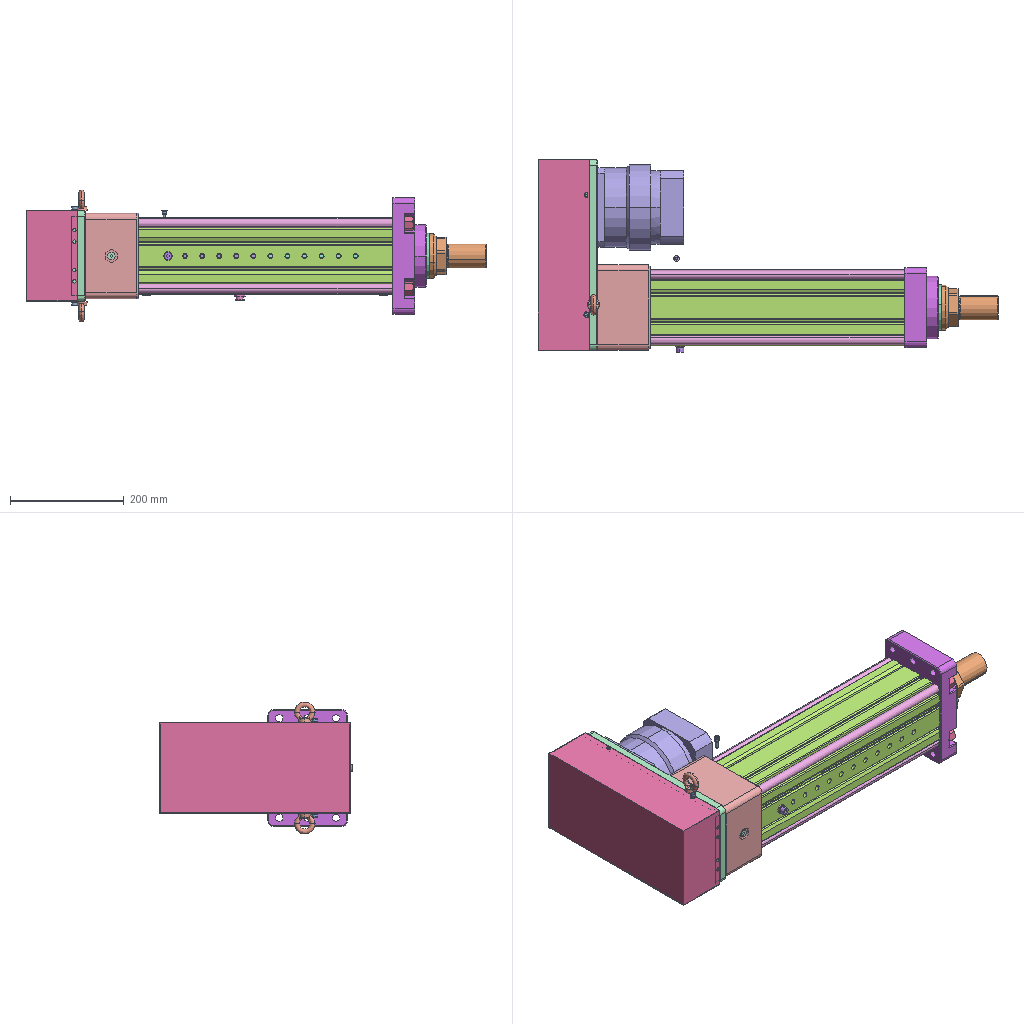Assembly | SolidWorks | 35 different items | 52 placed | box 809 x 339 x 232 mm
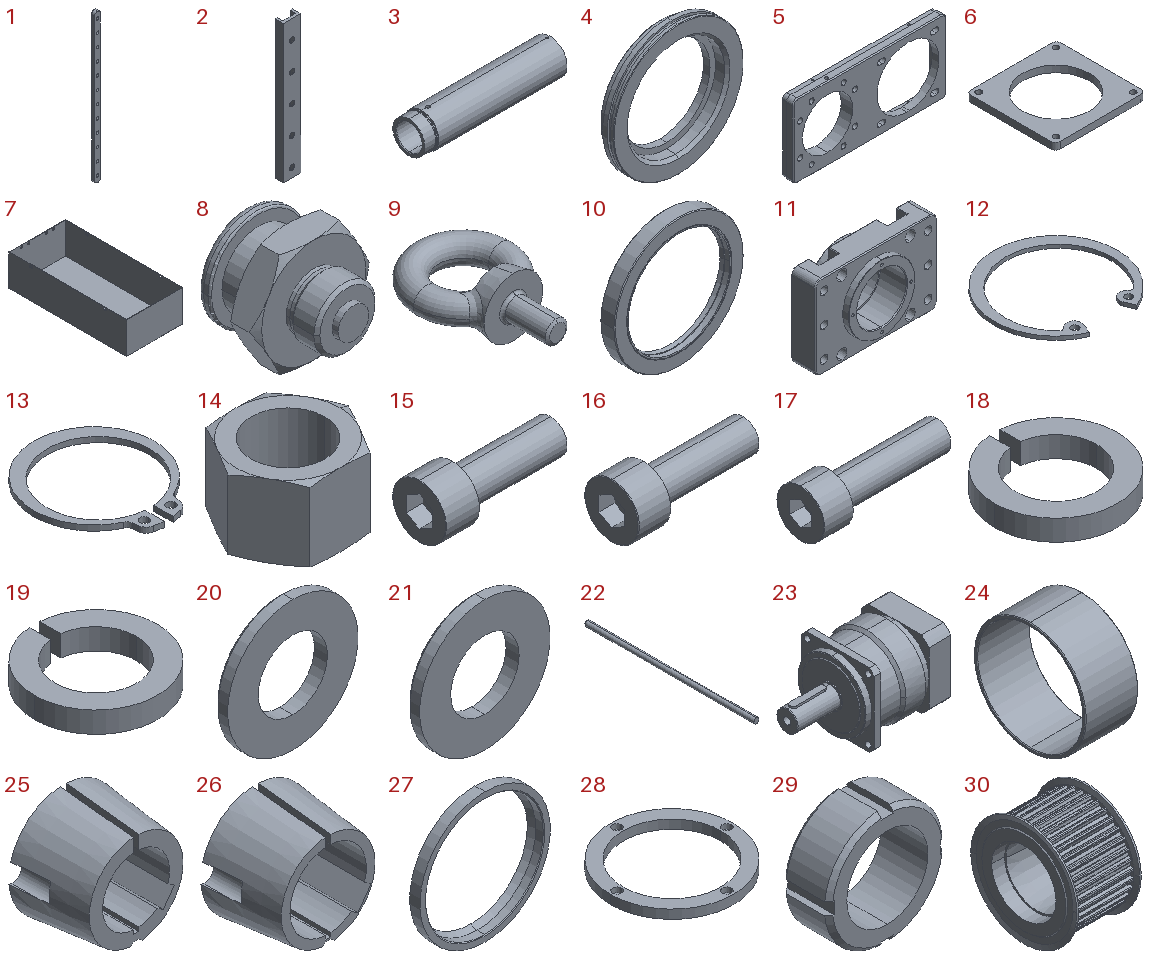Parts list (item | name | quantity | size | volume | features):
1 | - | x1 | 14 x 8 x 360 mm | 35757 mm3 | features ICE 2, Extrusion 1, Fillet 1, HoleWzd 1, LPattern 1
2 | - | x1 | 19 x 9 x 150 mm | 12195 mm3 | features Chamfer 1, Extrusion 1, HoleWzd 1, LPattern 1
3 | - | x1 | 330.5 x 80 x 80 mm | 682443 mm3 | features ICE 3, Chamfer 2, HoleWzd 1, Revolution 1
4 | - | x1 | 120 x 17 x 120 mm | 76412 mm3 | features ICE 4, Chamfer 3, Extrusion 1, MoveFace 1
5 | - | x1 | 335 x 25 x 160 mm | 627344 mm3 | features HoleWzd 7, ICE 6, MoveFace 4, Fillet 2, MirrorPattern 2, Chamfer 1, Extrusion 1
6 | - | x1 | 137 x 135 x 10 mm | 103302 mm3 | features HoleWzd 2, Extrusion 1, Fillet 1, ICE 1, MoveFace 1
7 | - | x1 | 160 x 335 x 90 mm | 168968 mm3 | features ICE 2, Extrusion 1, Shell 1
8 | - | x1 | 19.63 x 18 x 17 mm | 2444 mm3 | features ICE 3, Revolution 2
9 | - | x2 | 36.2 x 52.1 x 21.1 mm | 7704 mm3 | features Fillet 2, Extrusion 1, LPattern 1, RevCut 1, Revolution 1, Sweep 1
10 | - | x1 | 90 x 10 x 90 mm | 7063 mm3 | features BaseBody 1
11 | - | x1 | 205 x 70 x 140 mm | 920988 mm3 | features ICE 17, HoleWzd 12, Chamfer 11, Fillet 5, CirPattern 4, Extrusion 1, MirrorPattern 1, MoveFace 1, RevCut 1
12 | - | x1 | 50.5 x 48.578 x 1.5 mm | 759.16 mm3 | features Extrusion 1
13 | - | x1 | 27.3 x 30.557 x 1.2 mm | 213.948 mm3 | features Extrusion 1, Fillet 1
14 | - | x4 | 26.17 x 22.664 x 15.9 mm | 3864 mm3 | features Cut 2, Chamfer 1, Extrusion 1
15 | - | x2 | 40 x 16 x 16 mm | 4081 mm3 | features BlendCut 1, Cut 1, Fillet 1, LPattern 1, RevCut 1, Revolution 1
16 | - | x3 | 21 x 8.5 x 8.5 mm | 561.928 mm3 | features BlendCut 1, Cut 1, Fillet 1, LPattern 1, RevCut 1, Revolution 1
17 | - | x1 | 38 x 13 x 13 mm | 2440 mm3 | features BlendCut 1, Cut 1, Fillet 1, LPattern 1, RevCut 1, Revolution 1
18 | - | x3 | 7.686 x 7.672 x 1.3 mm | 32.664 mm3 | features Extrusion 1
19 | - | x1 | 12.277 x 12.254 x 2.1 mm | 135.755 mm3 | features Extrusion 1
20 | - | x3 | 10 x 1 x 10 mm | 55.513 mm3 | features Revolution 1
21 | - | x1 | 16 x 1.6 x 16 mm | 229.077 mm3 | features Revolution 1
22 | - | x4 | 16 x 531.5 x 16 mm | 106666 mm3 | features Chamfer 1, Extrusion 1
23 | - | x1 | 248.5 x 150 x 150 mm | 2601531 mm3 | features BaseBody 1
24 | - | x1 | 40 x 85 x 85 mm | 25789 mm3 | features Chamfer 3, MoveFace 1, Revolution 1
25 | - | x1 | 56.795 x 38 x 56.678 mm | 42357 mm3 | features BaseBody 1, ICE 1
26 | - | x1 | 56.795 x 38 x 56.678 mm | 31152 mm3 | features BaseBody 1, ICE 1
27 | - | x1 | 90 x 9.8 x 90 mm | 9491 mm3 | features Chamfer 1, Revolution 1
28 | - | x1 | 111 x 111 x 8 mm | 27617 mm3 | features CirPattern 1, Extrusion 1, HoleWzd 1
29 | - | x1 | 57.689 x 23 x 57.689 mm | 29622 mm3 | features Chamfer 1, CirPattern 1, Extrusion 1, ICE 1
30 | - | x2 | 60 x 99 x 99 mm | 224539 mm3 | features ICE 4, Revolution 2, Chamfer 1, CirPattern 1, MirrorPattern 1
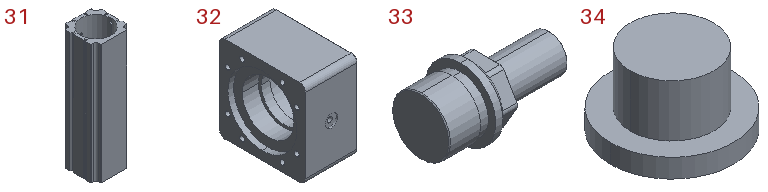31 | - | x1 | 134 x 134 x 446.5 mm | 2883696 mm3 | features ICE 6, HoleWzd 5, Chamfer 3, CirPattern 3, Fillet 3, LPattern 2, MirrorPattern 2, Extrusion 1, MoveFace 1
32 | - | x1 | 99 x 150 x 150 mm | 1431839 mm3 | features ICE 13, HoleWzd 4, Chamfer 2, CirPattern 1, Extrusion 1, Fillet 1
33 | - | x1 | 145 x 79 x 79 mm | 357004 mm3 | features ICE 7, Chamfer 6, Draft 2, Extrusion 1, Fillet 1, MoveFace 1
34 | - | x3 | 13 x 13 x 7.5 mm | 544.556 mm3 | features ICE 2, Extrusion 1
35 | hexagon socket countersunk head screws gb | x1 | - | - | -
Mates (type | each side: item.copy, entity, surface, feature):
Coincident | 32.1 plane | assembly plane | 2 times
Coincident | 32.1 face plane Boss-Extrude1 | 31.1 face plane Boss-Extrude1
Concentric | 32.1 face cylinder M16 Tapped Hole1 | 22.1 face cylinder Boss-Extrude1
Tangent | 31.1 face cylinder Boss-Extrude1 | 1.1 face plane Boss-Extrude1
Concentric | 31.1 face cylinder Ø9.0 (9) Diameter Hole1 | 1.1 face cylinder M8 Tapped Hole1
Coincident | 32.1 face plane Cut-Extrude9 | 28.1 face plane Boss-Extrude1
Concentric | 32.1 face cylinder M4 Tapped Hole2 | 28.1 face cylinder Hole size per socket head cap screw type 1
Concentric | 22.1 face cylinder Boss-Extrude1 | 14.1 face cylinder Base-Extrude
Concentric | 22.1 face cylinder Boss-Extrude1 | 11.1 face cylinder Hole size per socket head cap screw type 1
Coincident | 31.1 face plane Boss-Extrude1 | 11.1 face plane Boss-Extrude1
Concentric | 24.1 face cylinder Revolve1 | 11.1 face cylinder Cut-Extrude11
Coincident | 24.1 face plane Revolve1 | 11.1 face plane Cut-Extrude2
Concentric | 27.1 face cylinder Base-Revolve | 11.1 face cylinder Cut-Revolve2
Coincident | 27.1 face plane Base-Revolve | 11.1 face plane Cut-Revolve2
Concentric | 22.2 face cylinder Boss-Extrude1 | 11.1 face cylinder Hole size per socket head cap screw type 1
Coincident | 22.1 face plane Boss-Extrude1 | 22.2 face plane Boss-Extrude1
Concentric | 22.3 face cylinder Boss-Extrude1 | 11.1 face cylinder Hole size per socket head cap screw type 1
Coincident | 22.3 face plane Boss-Extrude1 | 11.1 face plane Boss-Extrude1
Concentric | 22.4 face cylinder Boss-Extrude1 | 11.1 face cylinder Hole size per socket head cap screw type 1
Coincident | 22.4 face plane Boss-Extrude1 | 11.1 face plane Boss-Extrude1
Coincident | 14.1 face plane Base-Extrude | 11.1 face plane Hole size per socket head cap screw type 1
Concentric | 32.1 face cylinder G1/8 Tapped Hole1 | 34.1 face cylinder Cut-Extrude1
Coincident | 32.1 face plane Cut-Extrude14 | 34.1 face plane Cut-Extrude1
Concentric | 25.1 face cylinder Input 1 | 30.1 face cone Cut-Extrude4
Coincident | 25.1 face plane Input 1 | 30.1 face plane Cut-Extrude3
Concentric | 31.1 face cylinder LPattern1 | 1.1 face cylinder LPattern1
Concentric | 31.1 face cylinder G1/8 Tapped Hole1 | 8.1 face cylinder Revolve1
Coincident | 31.1 face plane Boss-Extrude1 | 8.1 face plane Revolve1
Parallel | 32.1 face plane Boss-Extrude1 | 31.1 face plane Boss-Extrude1
Coincident | 31.1 face plane Boss-Extrude1 | assembly face
Coincident | 22.1 face plane Boss-Extrude1 | 22.4 face plane Boss-Extrude1
Concentric | 31.1 face cylinder G1/8 Tapped Hole2 | 34.2 face cylinder Cut-Extrude1
Coincident | 31.1 face plane Boss-Extrude1 | 34.2 face plane Cut-Extrude1
Concentric | 31.1 face cylinder G1/8 Tapped Hole2 | 34.3 face cylinder Cut-Extrude1
Coincident | 31.1 face plane Boss-Extrude1 | 34.3 face plane Cut-Extrude1
Concentric | 19.1 face cylinder Extrude1 | 21.1 face cylinder Base-Revolve
Coincident | 19.1 face plane Extrude1 | 21.1 face plane Base-Revolve
Concentric | 17.1 face cylinder Base-Revolve | 19.1 face cylinder Extrude1
Coincident | 17.1 edge | 19.1 face plane Extrude1
Concentric | 31.1 face cylinder Ø9.0 (9) Diameter Hole1 | 17.1 face cylinder Base-Revolve
Coincident | 31.1 face plane Boss-Extrude1 | 21.1 face plane Base-Revolve
Concentric | 18.1 face cylinder Extrude1 | 20.1 face cylinder Base-Revolve
Coincident | 18.1 face plane Extrude1 | 20.1 face plane Base-Revolve
Concentric | 16.1 face cylinder Base-Revolve | 18.1 face cylinder Extrude1
Coincident | 16.1 face plane Base-Revolve | 18.1 face plane Extrude1
Coincident | 32.1 face | assembly face
Coincident | assembly face | assembly face
Parallel | 31.1 face plane Boss-Extrude1 | 11.1 face plane Cut-Extrude15
Concentric | 3.1 face cylinder Cut-Extrude1 | 33.1 face cylinder Cut-Extrude3
Coincident | 3.1 face plane Revolve1 | 33.1 face plane Cut-Extrude3
LimitDistanceDim | 33.1 face plane Boss-Extrude1 | 11.1 face plane Boss-Extrude1
Width | 30.2 face plane Revolve2 | 30.2 face plane Revolve2 | 30.1 face plane Revolve2 | 30.1 face plane Revolve2
Concentric | 30.2 face cylinder Cut-Extrude3 | 26.1 face cylinder Input 1
Concentric | 23.1 face cylinder Input 1 | 26.1 face cylinder Input 1
Concentric | 23.1 face cylinder Input 1 | 6.1 face cylinder Cut-Extrude1
Parallel | 23.1 face plane Input 1 | 26.1 face plane Input 1
Coincident | 30.2 face plane Cut-Extrude3 | 26.1 face plane Input 1
Concentric | 32.1 face cylinder Cut-Extrude1 | 3.1 face cylinder Cut-Extrude2
Coincident | 20.1 face plane Base-Revolve | 7.1 face plane Boss-Extrude1
Concentric | 10.1 face cylinder Input 1 | 4.1 face cylinder Cut-Extrude3
Coincident | 32.1 face plane Cut-Extrude15 | 4.1 face plane Boss-Extrude1
Coincident | 10.1 face plane Input 1 | 4.1 face plane Cut-Extrude3
Concentric | 29.1 face cylinder Boss-Extrude1 | 5.1 face cylinder Cut-Extrude1
Coincident | 32.1 face plane Boss-Extrude1 | 5.1 face plane Boss-Extrude1
Coincident | 6.1 face plane Boss-Extrude1 | 5.1 face plane Cut-Extrude3
Slot | 6.1 face cylinder M10 Tapped Hole1 | 5.1 face cylinder Hole size per socket head cap screw type 29 | 2 times
Coincident | 23.1 face plane Input 1 | 5.1 face plane Boss-Extrude1
Coincident | 7.1 face plane Shell1 | 5.1 face plane Cut-Extrude4 | 2 times
Coincident | 7.1 face plane Boss-Extrude1 | 5.1 face plane Cut-Extrude4
Concentric | 32.1 face cylinder M10 Tapped Hole1 | 5.1 face cylinder Hole size per socket head cap screw type 11 | 2 times
Concentric | 9.1 face cylinder Base-Extrude | 5.1 face cylinder M8 Tapped Hole1
Coincident | 9.1 face plane Boss-Revolve1 | 5.1 face plane Boss-Extrude1
Concentric | 16.1 face cylinder Base-Revolve | 5.1 face cylinder Mirror1